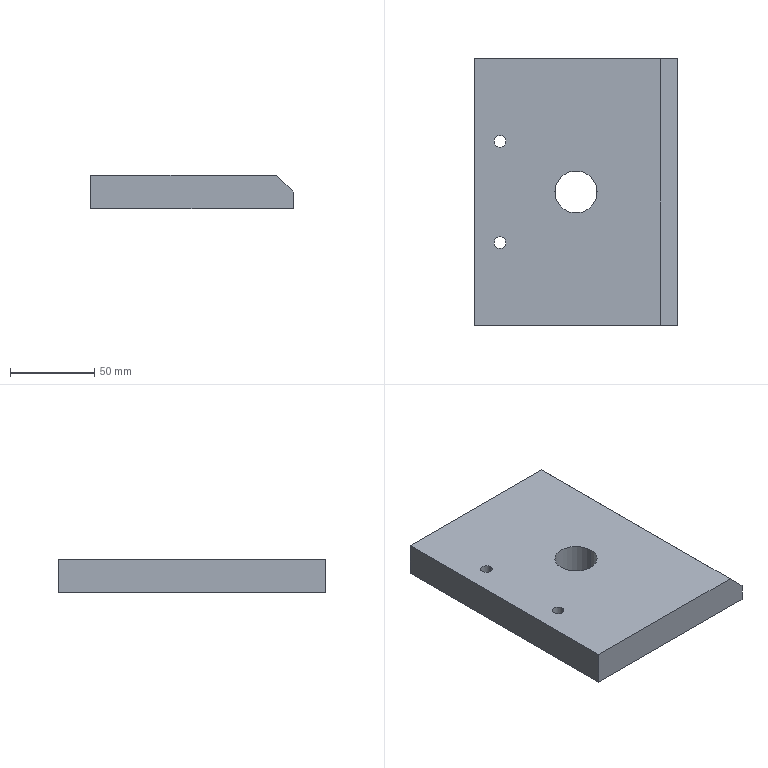Part | STEP file | 01-Top plate 1 | 1 solid | 13 faces | box 120 x 158 x 20 mm | volume 360030 mm3 | plane 7 | cylinder 6 | commonest cylinder face diameters 6.8 x4 25 x2
STEP:
#1=CARTESIAN_POINT('',(0.,0.,0.));
#2=DIRECTION('',(0.,0.,1.));
#3=DIRECTION('',(1.,0.,0.));
#4=AXIS2_PLACEMENT_3D('',#1,#2,#3);
#5=CARTESIAN_POINT('',(18.4,-49.,0.));
#6=VERTEX_POINT('',#5);
#7=CARTESIAN_POINT('',(18.4,-49.,20.));
#8=VERTEX_POINT('',#7);
#9=CARTESIAN_POINT('',(18.4,-49.,20.));
#10=DIRECTION('',(0.,0.,1.));
#11=VECTOR('',#10,1.);
#12=LINE('',#9,#11);
#13=CARTESIAN_POINT('',(15.,-49.,20.));
#14=DIRECTION('',(0.,0.,1.));
#15=DIRECTION('',(1.,0.,0.));
#16=AXIS2_PLACEMENT_3D('',#13,#14,#15);
#17=CYLINDRICAL_SURFACE('',#16,3.4);
#18=CARTESIAN_POINT('',(6.283,0.));
#19=DIRECTION('',(0.,1.));
#20=VECTOR('',#19,1.);
#21=LINE('',#18,#20);
#22=(GEOMETRIC_REPRESENTATION_CONTEXT(2)PARAMETRIC_REPRESENTATION_CONTEXT()REPRESENTATION_CONTEXT('',''));
#23=DEFINITIONAL_REPRESENTATION('',(#21),#22);
#24=PCURVE('',#17,#23);
#25=CARTESIAN_POINT('',(15.,-49.,20.));
#26=DIRECTION('',(0.,0.,1.));
#27=DIRECTION('',(1.,0.,0.));
#28=AXIS2_PLACEMENT_3D('',#25,#26,#27);
#29=CYLINDRICAL_SURFACE('',#28,3.4);
#30=CARTESIAN_POINT('',(0.,0.));
#31=DIRECTION('',(0.,1.));
#32=VECTOR('',#31,1.);
#33=LINE('',#30,#32);
#34=(GEOMETRIC_REPRESENTATION_CONTEXT(2)PARAMETRIC_REPRESENTATION_CONTEXT()REPRESENTATION_CONTEXT('',''));
#35=DEFINITIONAL_REPRESENTATION('',(#33),#34);
#36=PCURVE('',#29,#35);
#37=SURFACE_CURVE('',#12,(#24,#36),.PCURVE_S1.);
#38=EDGE_CURVE('',#6,#8,#37,.T.);
#39=ORIENTED_EDGE('',*,*,#38,.T.);
#40=CARTESIAN_POINT('',(11.6,-49.,20.));
#41=VERTEX_POINT('',#40);
#42=CARTESIAN_POINT('',(15.,-49.,20.));
#43=DIRECTION('',(0.,0.,1.));
#44=DIRECTION('',(1.,0.,0.));
#45=AXIS2_PLACEMENT_3D('',#42,#43,#44);
#46=CIRCLE('',#45,3.4);
#47=CARTESIAN_POINT('',(0.,0.));
#48=DIRECTION('',(1.,0.));
#49=VECTOR('',#48,1.);
#50=LINE('',#47,#49);
#51=(GEOMETRIC_REPRESENTATION_CONTEXT(2)PARAMETRIC_REPRESENTATION_CONTEXT()REPRESENTATION_CONTEXT('',''));
#52=DEFINITIONAL_REPRESENTATION('',(#50),#51);
#53=PCURVE('',#17,#52);
#54=CARTESIAN_POINT('',(0.,0.,20.));
#55=DIRECTION('',(0.,0.,1.));
#56=DIRECTION('',(1.,0.,0.));
#57=AXIS2_PLACEMENT_3D('',#54,#55,#56);
#58=PLANE('',#57);
#59=CARTESIAN_POINT('',(15.,-49.));
#60=DIRECTION('',(1.,0.));
#61=AXIS2_PLACEMENT_2D('',#59,#60);
#62=CIRCLE('',#61,3.4);
#63=(GEOMETRIC_REPRESENTATION_CONTEXT(2)PARAMETRIC_REPRESENTATION_CONTEXT()REPRESENTATION_CONTEXT('',''));
#64=DEFINITIONAL_REPRESENTATION('',(#62),#63);
#65=PCURVE('',#58,#64);
#66=SURFACE_CURVE('',#46,(#53,#65),.PCURVE_S1.);
#67=EDGE_CURVE('',#41,#8,#66,.T.);
#68=ORIENTED_EDGE('',*,*,#67,.F.);
#69=CARTESIAN_POINT('',(11.6,-49.,0.));
#70=VERTEX_POINT('',#69);
#71=CARTESIAN_POINT('',(11.6,-49.,20.));
#72=DIRECTION('',(0.,0.,1.));
#73=VECTOR('',#72,1.);
#74=LINE('',#71,#73);
#75=CARTESIAN_POINT('',(3.142,0.));
#76=DIRECTION('',(0.,1.));
#77=VECTOR('',#76,1.);
#78=LINE('',#75,#77);
#79=(GEOMETRIC_REPRESENTATION_CONTEXT(2)PARAMETRIC_REPRESENTATION_CONTEXT()REPRESENTATION_CONTEXT('',''));
#80=DEFINITIONAL_REPRESENTATION('',(#78),#79);
#81=PCURVE('',#17,#80);
#82=CARTESIAN_POINT('',(3.142,0.));
#83=DIRECTION('',(0.,1.));
#84=VECTOR('',#83,1.);
#85=LINE('',#82,#84);
#86=(GEOMETRIC_REPRESENTATION_CONTEXT(2)PARAMETRIC_REPRESENTATION_CONTEXT()REPRESENTATION_CONTEXT('',''));
#87=DEFINITIONAL_REPRESENTATION('',(#85),#86);
#88=PCURVE('',#29,#87);
#89=SURFACE_CURVE('',#74,(#81,#88),.PCURVE_S1.);
#90=EDGE_CURVE('',#70,#41,#89,.T.);
#91=ORIENTED_EDGE('',*,*,#90,.F.);
#92=CARTESIAN_POINT('',(15.,-49.,0.));
#93=DIRECTION('',(0.,0.,1.));
#94=DIRECTION('',(1.,0.,0.));
#95=AXIS2_PLACEMENT_3D('',#92,#93,#94);
#96=CIRCLE('',#95,3.4);
#97=CARTESIAN_POINT('',(0.,-20.));
#98=DIRECTION('',(1.,0.));
#99=VECTOR('',#98,1.);
#100=LINE('',#97,#99);
#101=(GEOMETRIC_REPRESENTATION_CONTEXT(2)PARAMETRIC_REPRESENTATION_CONTEXT()REPRESENTATION_CONTEXT('',''));
#102=DEFINITIONAL_REPRESENTATION('',(#100),#101);
#103=PCURVE('',#17,#102);
#104=CARTESIAN_POINT('',(0.,0.,0.));
#105=DIRECTION('',(0.,0.,1.));
#106=DIRECTION('',(1.,0.,0.));
#107=AXIS2_PLACEMENT_3D('',#104,#105,#106);
#108=PLANE('',#107);
#109=CARTESIAN_POINT('',(15.,-49.));
#110=DIRECTION('',(1.,0.));
#111=AXIS2_PLACEMENT_2D('',#109,#110);
#112=CIRCLE('',#111,3.4);
#113=(GEOMETRIC_REPRESENTATION_CONTEXT(2)PARAMETRIC_REPRESENTATION_CONTEXT()REPRESENTATION_CONTEXT('',''));
#114=DEFINITIONAL_REPRESENTATION('',(#112),#113);
#115=PCURVE('',#108,#114);
#116=SURFACE_CURVE('',#96,(#103,#115),.PCURVE_S1.);
#117=EDGE_CURVE('',#70,#6,#116,.T.);
#118=ORIENTED_EDGE('',*,*,#117,.T.);
#119=EDGE_LOOP('',(#39,#68,#91,#118));
#120=FACE_BOUND('',#119,.F.);
#121=ADVANCED_FACE('',(#120),#17,.F.);
#122=CARTESIAN_POINT('',(18.4,-109.,0.));
#123=VERTEX_POINT('',#122);
#124=CARTESIAN_POINT('',(18.4,-109.,20.));
#125=VERTEX_POINT('',#124);
#126=CARTESIAN_POINT('',(18.4,-109.,20.));
#127=DIRECTION('',(0.,0.,1.));
#128=VECTOR('',#127,1.);
#129=LINE('',#126,#128);
#130=CARTESIAN_POINT('',(15.,-109.,20.));
#131=DIRECTION('',(0.,0.,1.));
#132=DIRECTION('',(1.,0.,0.));
#133=AXIS2_PLACEMENT_3D('',#130,#131,#132);
#134=CYLINDRICAL_SURFACE('',#133,3.4);
#135=CARTESIAN_POINT('',(6.283,0.));
#136=DIRECTION('',(0.,1.));
#137=VECTOR('',#136,1.);
#138=LINE('',#135,#137);
#139=(GEOMETRIC_REPRESENTATION_CONTEXT(2)PARAMETRIC_REPRESENTATION_CONTEXT()REPRESENTATION_CONTEXT('',''));
#140=DEFINITIONAL_REPRESENTATION('',(#138),#139);
#141=PCURVE('',#134,#140);
#142=CARTESIAN_POINT('',(15.,-109.,20.));
#143=DIRECTION('',(0.,0.,1.));
#144=DIRECTION('',(1.,0.,0.));
#145=AXIS2_PLACEMENT_3D('',#142,#143,#144);
#146=CYLINDRICAL_SURFACE('',#145,3.4);
#147=CARTESIAN_POINT('',(0.,0.));
#148=DIRECTION('',(0.,1.));
#149=VECTOR('',#148,1.);
#150=LINE('',#147,#149);
#151=(GEOMETRIC_REPRESENTATION_CONTEXT(2)PARAMETRIC_REPRESENTATION_CONTEXT()REPRESENTATION_CONTEXT('',''));
#152=DEFINITIONAL_REPRESENTATION('',(#150),#151);
#153=PCURVE('',#146,#152);
#154=SURFACE_CURVE('',#129,(#141,#153),.PCURVE_S1.);
#155=EDGE_CURVE('',#123,#125,#154,.T.);
#156=ORIENTED_EDGE('',*,*,#155,.T.);
#157=CARTESIAN_POINT('',(11.6,-109.,20.));
#158=VERTEX_POINT('',#157);
#159=CARTESIAN_POINT('',(15.,-109.,20.));
#160=DIRECTION('',(0.,0.,1.));
#161=DIRECTION('',(1.,0.,0.));
#162=AXIS2_PLACEMENT_3D('',#159,#160,#161);
#163=CIRCLE('',#162,3.4);
#164=CARTESIAN_POINT('',(0.,0.));
#165=DIRECTION('',(1.,0.));
#166=VECTOR('',#165,1.);
#167=LINE('',#164,#166);
#168=(GEOMETRIC_REPRESENTATION_CONTEXT(2)PARAMETRIC_REPRESENTATION_CONTEXT()REPRESENTATION_CONTEXT('',''));
#169=DEFINITIONAL_REPRESENTATION('',(#167),#168);
#170=PCURVE('',#134,#169);
#171=CARTESIAN_POINT('',(15.,-109.));
#172=DIRECTION('',(1.,0.));
#173=AXIS2_PLACEMENT_2D('',#171,#172);
#174=CIRCLE('',#173,3.4);
#175=(GEOMETRIC_REPRESENTATION_CONTEXT(2)PARAMETRIC_REPRESENTATION_CONTEXT()REPRESENTATION_CONTEXT('',''));
#176=DEFINITIONAL_REPRESENTATION('',(#174),#175);
#177=PCURVE('',#58,#176);
#178=SURFACE_CURVE('',#163,(#170,#177),.PCURVE_S1.);
#179=EDGE_CURVE('',#158,#125,#178,.T.);
#180=ORIENTED_EDGE('',*,*,#179,.F.);
#181=CARTESIAN_POINT('',(11.6,-109.,0.));
#182=VERTEX_POINT('',#181);
#183=CARTESIAN_POINT('',(11.6,-109.,20.));
#184=DIRECTION('',(0.,0.,1.));
#185=VECTOR('',#184,1.);
#186=LINE('',#183,#185);
#187=CARTESIAN_POINT('',(3.142,0.));
#188=DIRECTION('',(0.,1.));
#189=VECTOR('',#188,1.);
#190=LINE('',#187,#189);
#191=(GEOMETRIC_REPRESENTATION_CONTEXT(2)PARAMETRIC_REPRESENTATION_CONTEXT()REPRESENTATION_CONTEXT('',''));
#192=DEFINITIONAL_REPRESENTATION('',(#190),#191);
#193=PCURVE('',#134,#192);
#194=CARTESIAN_POINT('',(3.142,0.));
#195=DIRECTION('',(0.,1.));
#196=VECTOR('',#195,1.);
#197=LINE('',#194,#196);
#198=(GEOMETRIC_REPRESENTATION_CONTEXT(2)PARAMETRIC_REPRESENTATION_CONTEXT()REPRESENTATION_CONTEXT('',''));
#199=DEFINITIONAL_REPRESENTATION('',(#197),#198);
#200=PCURVE('',#146,#199);
#201=SURFACE_CURVE('',#186,(#193,#200),.PCURVE_S1.);
#202=EDGE_CURVE('',#182,#158,#201,.T.);
#203=ORIENTED_EDGE('',*,*,#202,.F.);
#204=CARTESIAN_POINT('',(15.,-109.,0.));
#205=DIRECTION('',(0.,0.,1.));
#206=DIRECTION('',(1.,0.,0.));
#207=AXIS2_PLACEMENT_3D('',#204,#205,#206);
#208=CIRCLE('',#207,3.4);
#209=CARTESIAN_POINT('',(0.,-20.));
#210=DIRECTION('',(1.,0.));
#211=VECTOR('',#210,1.);
#212=LINE('',#209,#211);
#213=(GEOMETRIC_REPRESENTATION_CONTEXT(2)PARAMETRIC_REPRESENTATION_CONTEXT()REPRESENTATION_CONTEXT('',''));
#214=DEFINITIONAL_REPRESENTATION('',(#212),#213);
#215=PCURVE('',#134,#214);
#216=CARTESIAN_POINT('',(15.,-109.));
#217=DIRECTION('',(1.,0.));
#218=AXIS2_PLACEMENT_2D('',#216,#217);
#219=CIRCLE('',#218,3.4);
#220=(GEOMETRIC_REPRESENTATION_CONTEXT(2)PARAMETRIC_REPRESENTATION_CONTEXT()REPRESENTATION_CONTEXT('',''));
#221=DEFINITIONAL_REPRESENTATION('',(#219),#220);
#222=PCURVE('',#108,#221);
#223=SURFACE_CURVE('',#208,(#215,#222),.PCURVE_S1.);
#224=EDGE_CURVE('',#182,#123,#223,.T.);
#225=ORIENTED_EDGE('',*,*,#224,.T.);
#226=EDGE_LOOP('',(#156,#180,#203,#225));
#227=FACE_BOUND('',#226,.F.);
#228=ADVANCED_FACE('',(#227),#134,.F.);
#229=CARTESIAN_POINT('',(47.5,-79.,20.));
#230=VERTEX_POINT('',#229);
#231=CARTESIAN_POINT('',(47.5,-79.,0.));
#232=VERTEX_POINT('',#231);
#233=CARTESIAN_POINT('',(47.5,-79.,20.));
#234=DIRECTION('',(0.,0.,-1.));
#235=VECTOR('',#234,1.);
#236=LINE('',#233,#235);
#237=CARTESIAN_POINT('',(60.,-79.,20.));
#238=DIRECTION('',(0.,0.,-1.));
#239=DIRECTION('',(-1.,0.,0.));
#240=AXIS2_PLACEMENT_3D('',#237,#238,#239);
#241=CYLINDRICAL_SURFACE('',#240,12.5);
#242=CARTESIAN_POINT('',(6.283,0.));
#243=DIRECTION('',(0.,1.));
#244=VECTOR('',#243,1.);
#245=LINE('',#242,#244);
#246=(GEOMETRIC_REPRESENTATION_CONTEXT(2)PARAMETRIC_REPRESENTATION_CONTEXT()REPRESENTATION_CONTEXT('',''));
#247=DEFINITIONAL_REPRESENTATION('',(#245),#246);
#248=PCURVE('',#241,#247);
#249=CARTESIAN_POINT('',(60.,-79.,20.));
#250=DIRECTION('',(0.,0.,-1.));
#251=DIRECTION('',(-1.,0.,0.));
#252=AXIS2_PLACEMENT_3D('',#249,#250,#251);
#253=CYLINDRICAL_SURFACE('',#252,12.5);
#254=CARTESIAN_POINT('',(0.,0.));
#255=DIRECTION('',(0.,1.));
#256=VECTOR('',#255,1.);
#257=LINE('',#254,#256);
#258=(GEOMETRIC_REPRESENTATION_CONTEXT(2)PARAMETRIC_REPRESENTATION_CONTEXT()REPRESENTATION_CONTEXT('',''));
#259=DEFINITIONAL_REPRESENTATION('',(#257),#258);
#260=PCURVE('',#253,#259);
#261=SURFACE_CURVE('',#236,(#248,#260),.PCURVE_S1.);
#262=EDGE_CURVE('',#230,#232,#261,.T.);
#263=ORIENTED_EDGE('',*,*,#262,.T.);
#264=CARTESIAN_POINT('',(72.5,-79.,0.));
#265=VERTEX_POINT('',#264);
#266=CARTESIAN_POINT('',(60.,-79.,0.));
#267=DIRECTION('',(0.,0.,1.));
#268=DIRECTION('',(1.,0.,0.));
#269=AXIS2_PLACEMENT_3D('',#266,#267,#268);
#270=CIRCLE('',#269,12.5);
#271=CARTESIAN_POINT('',(9.425,20.));
#272=DIRECTION('',(-1.,0.));
#273=VECTOR('',#272,1.);
#274=LINE('',#271,#273);
#275=(GEOMETRIC_REPRESENTATION_CONTEXT(2)PARAMETRIC_REPRESENTATION_CONTEXT()REPRESENTATION_CONTEXT('',''));
#276=DEFINITIONAL_REPRESENTATION('',(#274),#275);
#277=PCURVE('',#241,#276);
#278=CARTESIAN_POINT('',(60.,-79.));
#279=DIRECTION('',(1.,0.));
#280=AXIS2_PLACEMENT_2D('',#278,#279);
#281=CIRCLE('',#280,12.5);
#282=(GEOMETRIC_REPRESENTATION_CONTEXT(2)PARAMETRIC_REPRESENTATION_CONTEXT()REPRESENTATION_CONTEXT('',''));
#283=DEFINITIONAL_REPRESENTATION('',(#281),#282);
#284=PCURVE('',#108,#283);
#285=SURFACE_CURVE('',#270,(#277,#284),.PCURVE_S1.);
#286=EDGE_CURVE('',#232,#265,#285,.T.);
#287=ORIENTED_EDGE('',*,*,#286,.T.);
#288=CARTESIAN_POINT('',(72.5,-79.,20.));
#289=VERTEX_POINT('',#288);
#290=CARTESIAN_POINT('',(72.5,-79.,20.));
#291=DIRECTION('',(0.,0.,-1.));
#292=VECTOR('',#291,1.);
#293=LINE('',#290,#292);
#294=CARTESIAN_POINT('',(3.142,0.));
#295=DIRECTION('',(0.,1.));
#296=VECTOR('',#295,1.);
#297=LINE('',#294,#296);
#298=(GEOMETRIC_REPRESENTATION_CONTEXT(2)PARAMETRIC_REPRESENTATION_CONTEXT()REPRESENTATION_CONTEXT('',''));
#299=DEFINITIONAL_REPRESENTATION('',(#297),#298);
#300=PCURVE('',#241,#299);
#301=CARTESIAN_POINT('',(3.142,0.));
#302=DIRECTION('',(0.,1.));
#303=VECTOR('',#302,1.);
#304=LINE('',#301,#303);
#305=(GEOMETRIC_REPRESENTATION_CONTEXT(2)PARAMETRIC_REPRESENTATION_CONTEXT()REPRESENTATION_CONTEXT('',''));
#306=DEFINITIONAL_REPRESENTATION('',(#304),#305);
#307=PCURVE('',#253,#306);
#308=SURFACE_CURVE('',#293,(#300,#307),.PCURVE_S1.);
#309=EDGE_CURVE('',#289,#265,#308,.T.);
#310=ORIENTED_EDGE('',*,*,#309,.F.);
#311=CARTESIAN_POINT('',(60.,-79.,20.));
#312=DIRECTION('',(0.,0.,1.));
#313=DIRECTION('',(1.,0.,0.));
#314=AXIS2_PLACEMENT_3D('',#311,#312,#313);
#315=CIRCLE('',#314,12.5);
#316=CARTESIAN_POINT('',(9.425,0.));
#317=DIRECTION('',(-1.,0.));
#318=VECTOR('',#317,1.);
#319=LINE('',#316,#318);
#320=(GEOMETRIC_REPRESENTATION_CONTEXT(2)PARAMETRIC_REPRESENTATION_CONTEXT()REPRESENTATION_CONTEXT('',''));
#321=DEFINITIONAL_REPRESENTATION('',(#319),#320);
#322=PCURVE('',#241,#321);
#323=CARTESIAN_POINT('',(60.,-79.));
#324=DIRECTION('',(1.,0.));
#325=AXIS2_PLACEMENT_2D('',#323,#324);
#326=CIRCLE('',#325,12.5);
#327=(GEOMETRIC_REPRESENTATION_CONTEXT(2)PARAMETRIC_REPRESENTATION_CONTEXT()REPRESENTATION_CONTEXT('',''));
#328=DEFINITIONAL_REPRESENTATION('',(#326),#327);
#329=PCURVE('',#58,#328);
#330=SURFACE_CURVE('',#315,(#322,#329),.PCURVE_S1.);
#331=EDGE_CURVE('',#230,#289,#330,.T.);
#332=ORIENTED_EDGE('',*,*,#331,.F.);
#333=EDGE_LOOP('',(#263,#287,#310,#332));
#334=FACE_BOUND('',#333,.F.);
#335=ADVANCED_FACE('',(#334),#241,.F.);
#336=CARTESIAN_POINT('',(15.,-49.,20.));
#337=DIRECTION('',(0.,0.,1.));
#338=DIRECTION('',(1.,0.,0.));
#339=AXIS2_PLACEMENT_3D('',#336,#337,#338);
#340=CIRCLE('',#339,3.4);
#341=CARTESIAN_POINT('',(15.,-49.));
#342=DIRECTION('',(1.,0.));
#343=AXIS2_PLACEMENT_2D('',#341,#342);
#344=CIRCLE('',#343,3.4);
#345=(GEOMETRIC_REPRESENTATION_CONTEXT(2)PARAMETRIC_REPRESENTATION_CONTEXT()REPRESENTATION_CONTEXT('',''));
#346=DEFINITIONAL_REPRESENTATION('',(#344),#345);
#347=PCURVE('',#58,#346);
#348=CARTESIAN_POINT('',(0.,0.));
#349=DIRECTION('',(1.,0.));
#350=VECTOR('',#349,1.);
#351=LINE('',#348,#350);
#352=(GEOMETRIC_REPRESENTATION_CONTEXT(2)PARAMETRIC_REPRESENTATION_CONTEXT()REPRESENTATION_CONTEXT('',''));
#353=DEFINITIONAL_REPRESENTATION('',(#351),#352);
#354=PCURVE('',#29,#353);
#355=SURFACE_CURVE('',#340,(#347,#354),.PCURVE_S1.);
#356=EDGE_CURVE('',#8,#41,#355,.T.);
#357=ORIENTED_EDGE('',*,*,#356,.F.);
#358=ORIENTED_EDGE('',*,*,#67,.F.);
#359=EDGE_LOOP('',(#357,#358));
#360=FACE_BOUND('',#359,.T.);
#361=CARTESIAN_POINT('',(15.,-109.,20.));
#362=DIRECTION('',(0.,0.,1.));
#363=DIRECTION('',(1.,0.,0.));
#364=AXIS2_PLACEMENT_3D('',#361,#362,#363);
#365=CIRCLE('',#364,3.4);
#366=CARTESIAN_POINT('',(15.,-109.));
#367=DIRECTION('',(1.,0.));
#368=AXIS2_PLACEMENT_2D('',#366,#367);
#369=CIRCLE('',#368,3.4);
#370=(GEOMETRIC_REPRESENTATION_CONTEXT(2)PARAMETRIC_REPRESENTATION_CONTEXT()REPRESENTATION_CONTEXT('',''));
#371=DEFINITIONAL_REPRESENTATION('',(#369),#370);
#372=PCURVE('',#58,#371);
#373=CARTESIAN_POINT('',(0.,0.));
#374=DIRECTION('',(1.,0.));
#375=VECTOR('',#374,1.);
#376=LINE('',#373,#375);
#377=(GEOMETRIC_REPRESENTATION_CONTEXT(2)PARAMETRIC_REPRESENTATION_CONTEXT()REPRESENTATION_CONTEXT('',''));
#378=DEFINITIONAL_REPRESENTATION('',(#376),#377);
#379=PCURVE('',#146,#378);
#380=SURFACE_CURVE('',#365,(#372,#379),.PCURVE_S1.);
#381=EDGE_CURVE('',#125,#158,#380,.T.);
#382=ORIENTED_EDGE('',*,*,#381,.F.);
#383=ORIENTED_EDGE('',*,*,#179,.F.);
#384=EDGE_LOOP('',(#382,#383));
#385=FACE_BOUND('',#384,.T.);
#386=CARTESIAN_POINT('',(0.,-158.,20.));
#387=VERTEX_POINT('',#386);
#388=CARTESIAN_POINT('',(110.,-158.,20.));
#389=VERTEX_POINT('',#388);
#390=CARTESIAN_POINT('',(0.,-158.,20.));
#391=DIRECTION('',(1.,0.,0.));
#392=VECTOR('',#391,1.);
#393=LINE('',#390,#392);
#394=CARTESIAN_POINT('',(0.,-158.));
#395=DIRECTION('',(1.,0.));
#396=VECTOR('',#395,1.);
#397=LINE('',#394,#396);
#398=(GEOMETRIC_REPRESENTATION_CONTEXT(2)PARAMETRIC_REPRESENTATION_CONTEXT()REPRESENTATION_CONTEXT('',''));
#399=DEFINITIONAL_REPRESENTATION('',(#397),#398);
#400=PCURVE('',#58,#399);
#401=CARTESIAN_POINT('',(0.,-158.,20.));
#402=DIRECTION('',(0.,1.,0.));
#403=DIRECTION('',(0.,0.,1.));
#404=AXIS2_PLACEMENT_3D('',#401,#402,#403);
#405=PLANE('',#404);
#406=CARTESIAN_POINT('',(0.,0.));
#407=DIRECTION('',(0.,1.));
#408=VECTOR('',#407,1.);
#409=LINE('',#406,#408);
#410=(GEOMETRIC_REPRESENTATION_CONTEXT(2)PARAMETRIC_REPRESENTATION_CONTEXT()REPRESENTATION_CONTEXT('',''));
#411=DEFINITIONAL_REPRESENTATION('',(#409),#410);
#412=PCURVE('',#405,#411);
#413=SURFACE_CURVE('',#393,(#400,#412),.PCURVE_S1.);
#414=EDGE_CURVE('',#387,#389,#413,.T.);
#415=ORIENTED_EDGE('',*,*,#414,.T.);
#416=CARTESIAN_POINT('',(110.,0.,20.));
#417=VERTEX_POINT('',#416);
#418=CARTESIAN_POINT('',(110.,0.,20.));
#419=DIRECTION('',(0.,1.,0.));
#420=VECTOR('',#419,1.);
#421=LINE('',#418,#420);
#422=CARTESIAN_POINT('',(110.,0.));
#423=DIRECTION('',(0.,1.));
#424=VECTOR('',#423,1.);
#425=LINE('',#422,#424);
#426=(GEOMETRIC_REPRESENTATION_CONTEXT(2)PARAMETRIC_REPRESENTATION_CONTEXT()REPRESENTATION_CONTEXT('',''));
#427=DEFINITIONAL_REPRESENTATION('',(#425),#426);
#428=PCURVE('',#58,#427);
#429=CARTESIAN_POINT('',(110.,0.,20.));
#430=DIRECTION('',(0.7071,0.,0.7071));
#431=DIRECTION('',(0.,-1.,0.));
#432=AXIS2_PLACEMENT_3D('',#429,#430,#431);
#433=PLANE('',#432);
#434=CARTESIAN_POINT('',(0.,0.));
#435=DIRECTION('',(-1.,0.));
#436=VECTOR('',#435,1.);
#437=LINE('',#434,#436);
#438=(GEOMETRIC_REPRESENTATION_CONTEXT(2)PARAMETRIC_REPRESENTATION_CONTEXT()REPRESENTATION_CONTEXT('',''));
#439=DEFINITIONAL_REPRESENTATION('',(#437),#438);
#440=PCURVE('',#433,#439);
#441=SURFACE_CURVE('',#421,(#428,#440),.PCURVE_S1.);
#442=EDGE_CURVE('',#389,#417,#441,.T.);
#443=ORIENTED_EDGE('',*,*,#442,.T.);
#444=CARTESIAN_POINT('',(0.,0.,20.));
#445=VERTEX_POINT('',#444);
#446=CARTESIAN_POINT('',(0.,0.,20.));
#447=DIRECTION('',(-1.,0.,0.));
#448=VECTOR('',#447,1.);
#449=LINE('',#446,#448);
#450=CARTESIAN_POINT('',(0.,0.));
#451=DIRECTION('',(-1.,0.));
#452=VECTOR('',#451,1.);
#453=LINE('',#450,#452);
#454=(GEOMETRIC_REPRESENTATION_CONTEXT(2)PARAMETRIC_REPRESENTATION_CONTEXT()REPRESENTATION_CONTEXT('',''));
#455=DEFINITIONAL_REPRESENTATION('',(#453),#454);
#456=PCURVE('',#58,#455);
#457=CARTESIAN_POINT('',(0.,0.,20.));
#458=DIRECTION('',(0.,-1.,0.));
#459=DIRECTION('',(0.,0.,-1.));
#460=AXIS2_PLACEMENT_3D('',#457,#458,#459);
#461=PLANE('',#460);
#462=CARTESIAN_POINT('',(0.,0.));
#463=DIRECTION('',(0.,-1.));
#464=VECTOR('',#463,1.);
#465=LINE('',#462,#464);
#466=(GEOMETRIC_REPRESENTATION_CONTEXT(2)PARAMETRIC_REPRESENTATION_CONTEXT()REPRESENTATION_CONTEXT('',''));
#467=DEFINITIONAL_REPRESENTATION('',(#465),#466);
#468=PCURVE('',#461,#467);
#469=SURFACE_CURVE('',#449,(#456,#468),.PCURVE_S1.);
#470=EDGE_CURVE('',#417,#445,#469,.T.);
#471=ORIENTED_EDGE('',*,*,#470,.T.);
#472=CARTESIAN_POINT('',(0.,0.,20.));
#473=DIRECTION('',(0.,-1.,0.));
#474=VECTOR('',#473,1.);
#475=LINE('',#472,#474);
#476=CARTESIAN_POINT('',(0.,0.));
#477=DIRECTION('',(0.,-1.));
#478=VECTOR('',#477,1.);
#479=LINE('',#476,#478);
#480=(GEOMETRIC_REPRESENTATION_CONTEXT(2)PARAMETRIC_REPRESENTATION_CONTEXT()REPRESENTATION_CONTEXT('',''));
#481=DEFINITIONAL_REPRESENTATION('',(#479),#480);
#482=PCURVE('',#58,#481);
#483=CARTESIAN_POINT('',(0.,0.,20.));
#484=DIRECTION('',(1.,0.,0.));
#485=DIRECTION('',(0.,1.,0.));
#486=AXIS2_PLACEMENT_3D('',#483,#484,#485);
#487=PLANE('',#486);
#488=CARTESIAN_POINT('',(0.,0.));
#489=DIRECTION('',(-1.,0.));
#490=VECTOR('',#489,1.);
#491=LINE('',#488,#490);
#492=(GEOMETRIC_REPRESENTATION_CONTEXT(2)PARAMETRIC_REPRESENTATION_CONTEXT()REPRESENTATION_CONTEXT('',''));
#493=DEFINITIONAL_REPRESENTATION('',(#491),#492);
#494=PCURVE('',#487,#493);
#495=SURFACE_CURVE('',#475,(#482,#494),.PCURVE_S1.);
#496=EDGE_CURVE('',#445,#387,#495,.T.);
#497=ORIENTED_EDGE('',*,*,#496,.T.);
#498=EDGE_LOOP('',(#415,#443,#471,#497));
#499=FACE_BOUND('',#498,.T.);
#500=ORIENTED_EDGE('',*,*,#331,.F.);
#501=CARTESIAN_POINT('',(60.,-79.,20.));
#502=DIRECTION('',(0.,0.,1.));
#503=DIRECTION('',(1.,0.,0.));
#504=AXIS2_PLACEMENT_3D('',#501,#502,#503);
#505=CIRCLE('',#504,12.5);
#506=CARTESIAN_POINT('',(60.,-79.));
#507=DIRECTION('',(1.,0.));
#508=AXIS2_PLACEMENT_2D('',#506,#507);
#509=CIRCLE('',#508,12.5);
#510=(GEOMETRIC_REPRESENTATION_CONTEXT(2)PARAMETRIC_REPRESENTATION_CONTEXT()REPRESENTATION_CONTEXT('',''));
#511=DEFINITIONAL_REPRESENTATION('',(#509),#510);
#512=PCURVE('',#58,#511);
#513=CARTESIAN_POINT('',(3.142,0.));
#514=DIRECTION('',(-1.,0.));
#515=VECTOR('',#514,1.);
#516=LINE('',#513,#515);
#517=(GEOMETRIC_REPRESENTATION_CONTEXT(2)PARAMETRIC_REPRESENTATION_CONTEXT()REPRESENTATION_CONTEXT('',''));
#518=DEFINITIONAL_REPRESENTATION('',(#516),#517);
#519=PCURVE('',#253,#518);
#520=SURFACE_CURVE('',#505,(#512,#519),.PCURVE_S1.);
#521=EDGE_CURVE('',#289,#230,#520,.T.);
#522=ORIENTED_EDGE('',*,*,#521,.F.);
#523=EDGE_LOOP('',(#500,#522));
#524=FACE_BOUND('',#523,.T.);
#525=ADVANCED_FACE('',(#360,#385,#499,#524),#58,.T.);
#526=CARTESIAN_POINT('',(15.,-49.,0.));
#527=DIRECTION('',(0.,0.,1.));
#528=DIRECTION('',(1.,0.,0.));
#529=AXIS2_PLACEMENT_3D('',#526,#527,#528);
#530=CIRCLE('',#529,3.4);
#531=CARTESIAN_POINT('',(15.,-49.));
#532=DIRECTION('',(1.,0.));
#533=AXIS2_PLACEMENT_2D('',#531,#532);
#534=CIRCLE('',#533,3.4);
#535=(GEOMETRIC_REPRESENTATION_CONTEXT(2)PARAMETRIC_REPRESENTATION_CONTEXT()REPRESENTATION_CONTEXT('',''));
#536=DEFINITIONAL_REPRESENTATION('',(#534),#535);
#537=PCURVE('',#108,#536);
#538=CARTESIAN_POINT('',(0.,-20.));
#539=DIRECTION('',(1.,0.));
#540=VECTOR('',#539,1.);
#541=LINE('',#538,#540);
#542=(GEOMETRIC_REPRESENTATION_CONTEXT(2)PARAMETRIC_REPRESENTATION_CONTEXT()REPRESENTATION_CONTEXT('',''));
#543=DEFINITIONAL_REPRESENTATION('',(#541),#542);
#544=PCURVE('',#29,#543);
#545=SURFACE_CURVE('',#530,(#537,#544),.PCURVE_S1.);
#546=EDGE_CURVE('',#6,#70,#545,.T.);
#547=ORIENTED_EDGE('',*,*,#546,.T.);
#548=ORIENTED_EDGE('',*,*,#117,.T.);
#549=EDGE_LOOP('',(#547,#548));
#550=FACE_BOUND('',#549,.T.);
#551=CARTESIAN_POINT('',(15.,-109.,0.));
#552=DIRECTION('',(0.,0.,1.));
#553=DIRECTION('',(1.,0.,0.));
#554=AXIS2_PLACEMENT_3D('',#551,#552,#553);
#555=CIRCLE('',#554,3.4);
#556=CARTESIAN_POINT('',(15.,-109.));
#557=DIRECTION('',(1.,0.));
#558=AXIS2_PLACEMENT_2D('',#556,#557);
#559=CIRCLE('',#558,3.4);
#560=(GEOMETRIC_REPRESENTATION_CONTEXT(2)PARAMETRIC_REPRESENTATION_CONTEXT()REPRESENTATION_CONTEXT('',''));
#561=DEFINITIONAL_REPRESENTATION('',(#559),#560);
#562=PCURVE('',#108,#561);
#563=CARTESIAN_POINT('',(0.,-20.));
#564=DIRECTION('',(1.,0.));
#565=VECTOR('',#564,1.);
#566=LINE('',#563,#565);
#567=(GEOMETRIC_REPRESENTATION_CONTEXT(2)PARAMETRIC_REPRESENTATION_CONTEXT()REPRESENTATION_CONTEXT('',''));
#568=DEFINITIONAL_REPRESENTATION('',(#566),#567);
#569=PCURVE('',#146,#568);
#570=SURFACE_CURVE('',#555,(#562,#569),.PCURVE_S1.);
#571=EDGE_CURVE('',#123,#182,#570,.T.);
#572=ORIENTED_EDGE('',*,*,#571,.T.);
#573=ORIENTED_EDGE('',*,*,#224,.T.);
#574=EDGE_LOOP('',(#572,#573));
#575=FACE_BOUND('',#574,.T.);
#576=CARTESIAN_POINT('',(0.,0.,0.));
#577=VERTEX_POINT('',#576);
#578=CARTESIAN_POINT('',(0.,-158.,0.));
#579=VERTEX_POINT('',#578);
#580=CARTESIAN_POINT('',(0.,0.,0.));
#581=DIRECTION('',(0.,-1.,0.));
#582=VECTOR('',#581,1.);
#583=LINE('',#580,#582);
#584=CARTESIAN_POINT('',(0.,0.));
#585=DIRECTION('',(0.,-1.));
#586=VECTOR('',#585,1.);
#587=LINE('',#584,#586);
#588=(GEOMETRIC_REPRESENTATION_CONTEXT(2)PARAMETRIC_REPRESENTATION_CONTEXT()REPRESENTATION_CONTEXT('',''));
#589=DEFINITIONAL_REPRESENTATION('',(#587),#588);
#590=PCURVE('',#108,#589);
#591=CARTESIAN_POINT('',(0.,-20.));
#592=DIRECTION('',(-1.,0.));
#593=VECTOR('',#592,1.);
#594=LINE('',#591,#593);
#595=(GEOMETRIC_REPRESENTATION_CONTEXT(2)PARAMETRIC_REPRESENTATION_CONTEXT()REPRESENTATION_CONTEXT('',''));
#596=DEFINITIONAL_REPRESENTATION('',(#594),#595);
#597=PCURVE('',#487,#596);
#598=SURFACE_CURVE('',#583,(#590,#597),.PCURVE_S1.);
#599=EDGE_CURVE('',#577,#579,#598,.T.);
#600=ORIENTED_EDGE('',*,*,#599,.F.);
#601=CARTESIAN_POINT('',(120.,0.,0.));
#602=VERTEX_POINT('',#601);
#603=CARTESIAN_POINT('',(0.,0.,0.));
#604=DIRECTION('',(-1.,0.,0.));
#605=VECTOR('',#604,1.);
#606=LINE('',#603,#605);
#607=CARTESIAN_POINT('',(0.,0.));
#608=DIRECTION('',(-1.,0.));
#609=VECTOR('',#608,1.);
#610=LINE('',#607,#609);
#611=(GEOMETRIC_REPRESENTATION_CONTEXT(2)PARAMETRIC_REPRESENTATION_CONTEXT()REPRESENTATION_CONTEXT('',''));
#612=DEFINITIONAL_REPRESENTATION('',(#610),#611);
#613=PCURVE('',#108,#612);
#614=CARTESIAN_POINT('',(20.,0.));
#615=DIRECTION('',(0.,-1.));
#616=VECTOR('',#615,1.);
#617=LINE('',#614,#616);
#618=(GEOMETRIC_REPRESENTATION_CONTEXT(2)PARAMETRIC_REPRESENTATION_CONTEXT()REPRESENTATION_CONTEXT('',''));
#619=DEFINITIONAL_REPRESENTATION('',(#617),#618);
#620=PCURVE('',#461,#619);
#621=SURFACE_CURVE('',#606,(#613,#620),.PCURVE_S1.);
#622=EDGE_CURVE('',#602,#577,#621,.T.);
#623=ORIENTED_EDGE('',*,*,#622,.F.);
#624=CARTESIAN_POINT('',(120.,-158.,0.));
#625=VERTEX_POINT('',#624);
#626=CARTESIAN_POINT('',(120.,0.,0.));
#627=DIRECTION('',(0.,1.,0.));
#628=VECTOR('',#627,1.);
#629=LINE('',#626,#628);
#630=CARTESIAN_POINT('',(120.,0.));
#631=DIRECTION('',(0.,1.));
#632=VECTOR('',#631,1.);
#633=LINE('',#630,#632);
#634=(GEOMETRIC_REPRESENTATION_CONTEXT(2)PARAMETRIC_REPRESENTATION_CONTEXT()REPRESENTATION_CONTEXT('',''));
#635=DEFINITIONAL_REPRESENTATION('',(#633),#634);
#636=PCURVE('',#108,#635);
#637=CARTESIAN_POINT('',(120.,0.,20.));
#638=DIRECTION('',(-1.,0.,0.));
#639=DIRECTION('',(0.,-1.,0.));
#640=AXIS2_PLACEMENT_3D('',#637,#638,#639);
#641=PLANE('',#640);
#642=CARTESIAN_POINT('',(0.,-20.));
#643=DIRECTION('',(-1.,0.));
#644=VECTOR('',#643,1.);
#645=LINE('',#642,#644);
#646=(GEOMETRIC_REPRESENTATION_CONTEXT(2)PARAMETRIC_REPRESENTATION_CONTEXT()REPRESENTATION_CONTEXT('',''));
#647=DEFINITIONAL_REPRESENTATION('',(#645),#646);
#648=PCURVE('',#641,#647);
#649=SURFACE_CURVE('',#629,(#636,#648),.PCURVE_S1.);
#650=EDGE_CURVE('',#625,#602,#649,.T.);
#651=ORIENTED_EDGE('',*,*,#650,.F.);
#652=CARTESIAN_POINT('',(0.,-158.,0.));
#653=DIRECTION('',(1.,0.,0.));
#654=VECTOR('',#653,1.);
#655=LINE('',#652,#654);
#656=CARTESIAN_POINT('',(0.,-158.));
#657=DIRECTION('',(1.,0.));
#658=VECTOR('',#657,1.);
#659=LINE('',#656,#658);
#660=(GEOMETRIC_REPRESENTATION_CONTEXT(2)PARAMETRIC_REPRESENTATION_CONTEXT()REPRESENTATION_CONTEXT('',''));
#661=DEFINITIONAL_REPRESENTATION('',(#659),#660);
#662=PCURVE('',#108,#661);
#663=CARTESIAN_POINT('',(-20.,0.));
#664=DIRECTION('',(0.,1.));
#665=VECTOR('',#664,1.);
#666=LINE('',#663,#665);
#667=(GEOMETRIC_REPRESENTATION_CONTEXT(2)PARAMETRIC_REPRESENTATION_CONTEXT()REPRESENTATION_CONTEXT('',''));
#668=DEFINITIONAL_REPRESENTATION('',(#666),#667);
#669=PCURVE('',#405,#668);
#670=SURFACE_CURVE('',#655,(#662,#669),.PCURVE_S1.);
#671=EDGE_CURVE('',#579,#625,#670,.T.);
#672=ORIENTED_EDGE('',*,*,#671,.F.);
#673=EDGE_LOOP('',(#600,#623,#651,#672));
#674=FACE_BOUND('',#673,.T.);
#675=ORIENTED_EDGE('',*,*,#286,.T.);
#676=CARTESIAN_POINT('',(60.,-79.,0.));
#677=DIRECTION('',(0.,0.,1.));
#678=DIRECTION('',(1.,0.,0.));
#679=AXIS2_PLACEMENT_3D('',#676,#677,#678);
#680=CIRCLE('',#679,12.5);
#681=CARTESIAN_POINT('',(60.,-79.));
#682=DIRECTION('',(1.,0.));
#683=AXIS2_PLACEMENT_2D('',#681,#682);
#684=CIRCLE('',#683,12.5);
#685=(GEOMETRIC_REPRESENTATION_CONTEXT(2)PARAMETRIC_REPRESENTATION_CONTEXT()REPRESENTATION_CONTEXT('',''));
#686=DEFINITIONAL_REPRESENTATION('',(#684),#685);
#687=PCURVE('',#108,#686);
#688=CARTESIAN_POINT('',(3.142,20.));
#689=DIRECTION('',(-1.,0.));
#690=VECTOR('',#689,1.);
#691=LINE('',#688,#690);
#692=(GEOMETRIC_REPRESENTATION_CONTEXT(2)PARAMETRIC_REPRESENTATION_CONTEXT()REPRESENTATION_CONTEXT('',''));
#693=DEFINITIONAL_REPRESENTATION('',(#691),#692);
#694=PCURVE('',#253,#693);
#695=SURFACE_CURVE('',#680,(#687,#694),.PCURVE_S1.);
#696=EDGE_CURVE('',#265,#232,#695,.T.);
#697=ORIENTED_EDGE('',*,*,#696,.T.);
#698=EDGE_LOOP('',(#675,#697));
#699=FACE_BOUND('',#698,.T.);
#700=ADVANCED_FACE('',(#550,#575,#674,#699),#108,.F.);
#701=ORIENTED_EDGE('',*,*,#599,.T.);
#702=CARTESIAN_POINT('',(0.,-158.,20.));
#703=DIRECTION('',(0.,0.,-1.));
#704=VECTOR('',#703,1.);
#705=LINE('',#702,#704);
#706=CARTESIAN_POINT('',(-158.,0.));
#707=DIRECTION('',(0.,-1.));
#708=VECTOR('',#707,1.);
#709=LINE('',#706,#708);
#710=(GEOMETRIC_REPRESENTATION_CONTEXT(2)PARAMETRIC_REPRESENTATION_CONTEXT()REPRESENTATION_CONTEXT('',''));
#711=DEFINITIONAL_REPRESENTATION('',(#709),#710);
#712=PCURVE('',#487,#711);
#713=CARTESIAN_POINT('',(0.,0.));
#714=DIRECTION('',(-1.,0.));
#715=VECTOR('',#714,1.);
#716=LINE('',#713,#715);
#717=(GEOMETRIC_REPRESENTATION_CONTEXT(2)PARAMETRIC_REPRESENTATION_CONTEXT()REPRESENTATION_CONTEXT('',''));
#718=DEFINITIONAL_REPRESENTATION('',(#716),#717);
#719=PCURVE('',#405,#718);
#720=SURFACE_CURVE('',#705,(#712,#719),.PCURVE_S1.);
#721=EDGE_CURVE('',#387,#579,#720,.T.);
#722=ORIENTED_EDGE('',*,*,#721,.F.);
#723=ORIENTED_EDGE('',*,*,#496,.F.);
#724=CARTESIAN_POINT('',(0.,0.,20.));
#725=DIRECTION('',(0.,0.,-1.));
#726=VECTOR('',#725,1.);
#727=LINE('',#724,#726);
#728=CARTESIAN_POINT('',(0.,0.));
#729=DIRECTION('',(0.,-1.));
#730=VECTOR('',#729,1.);
#731=LINE('',#728,#730);
#732=(GEOMETRIC_REPRESENTATION_CONTEXT(2)PARAMETRIC_REPRESENTATION_CONTEXT()REPRESENTATION_CONTEXT('',''));
#733=DEFINITIONAL_REPRESENTATION('',(#731),#732);
#734=PCURVE('',#487,#733);
#735=CARTESIAN_POINT('',(0.,0.));
#736=DIRECTION('',(1.,0.));
#737=VECTOR('',#736,1.);
#738=LINE('',#735,#737);
#739=(GEOMETRIC_REPRESENTATION_CONTEXT(2)PARAMETRIC_REPRESENTATION_CONTEXT()REPRESENTATION_CONTEXT('',''));
#740=DEFINITIONAL_REPRESENTATION('',(#738),#739);
#741=PCURVE('',#461,#740);
#742=SURFACE_CURVE('',#727,(#734,#741),.PCURVE_S1.);
#743=EDGE_CURVE('',#445,#577,#742,.T.);
#744=ORIENTED_EDGE('',*,*,#743,.T.);
#745=EDGE_LOOP('',(#701,#722,#723,#744));
#746=FACE_BOUND('',#745,.T.);
#747=ADVANCED_FACE('',(#746),#487,.F.);
#748=CARTESIAN_POINT('',(120.,-158.,10.));
#749=VERTEX_POINT('',#748);
#750=CARTESIAN_POINT('',(120.,-158.,20.));
#751=DIRECTION('',(0.,0.,-1.));
#752=VECTOR('',#751,1.);
#753=LINE('',#750,#752);
#754=CARTESIAN_POINT('',(0.,120.));
#755=DIRECTION('',(-1.,0.));
#756=VECTOR('',#755,1.);
#757=LINE('',#754,#756);
#758=(GEOMETRIC_REPRESENTATION_CONTEXT(2)PARAMETRIC_REPRESENTATION_CONTEXT()REPRESENTATION_CONTEXT('',''));
#759=DEFINITIONAL_REPRESENTATION('',(#757),#758);
#760=PCURVE('',#405,#759);
#761=CARTESIAN_POINT('',(158.,0.));
#762=DIRECTION('',(0.,-1.));
#763=VECTOR('',#762,1.);
#764=LINE('',#761,#763);
#765=(GEOMETRIC_REPRESENTATION_CONTEXT(2)PARAMETRIC_REPRESENTATION_CONTEXT()REPRESENTATION_CONTEXT('',''));
#766=DEFINITIONAL_REPRESENTATION('',(#764),#765);
#767=PCURVE('',#641,#766);
#768=SURFACE_CURVE('',#753,(#760,#767),.PCURVE_S1.);
#769=EDGE_CURVE('',#749,#625,#768,.T.);
#770=ORIENTED_EDGE('',*,*,#769,.F.);
#771=CARTESIAN_POINT('',(110.,-158.,20.));
#772=DIRECTION('',(-0.7071,0.,0.7071));
#773=VECTOR('',#772,1.);
#774=LINE('',#771,#773);
#775=CARTESIAN_POINT('',(0.,110.));
#776=DIRECTION('',(0.7071,-0.7071));
#777=VECTOR('',#776,1.);
#778=LINE('',#775,#777);
#779=(GEOMETRIC_REPRESENTATION_CONTEXT(2)PARAMETRIC_REPRESENTATION_CONTEXT()REPRESENTATION_CONTEXT('',''));
#780=DEFINITIONAL_REPRESENTATION('',(#778),#779);
#781=PCURVE('',#405,#780);
#782=CARTESIAN_POINT('',(158.,0.));
#783=DIRECTION('',(0.,-1.));
#784=VECTOR('',#783,1.);
#785=LINE('',#782,#784);
#786=(GEOMETRIC_REPRESENTATION_CONTEXT(2)PARAMETRIC_REPRESENTATION_CONTEXT()REPRESENTATION_CONTEXT('',''));
#787=DEFINITIONAL_REPRESENTATION('',(#785),#786);
#788=PCURVE('',#433,#787);
#789=SURFACE_CURVE('',#774,(#781,#788),.PCURVE_S1.);
#790=EDGE_CURVE('',#749,#389,#789,.T.);
#791=ORIENTED_EDGE('',*,*,#790,.T.);
#792=ORIENTED_EDGE('',*,*,#414,.F.);
#793=ORIENTED_EDGE('',*,*,#721,.T.);
#794=ORIENTED_EDGE('',*,*,#671,.T.);
#795=EDGE_LOOP('',(#770,#791,#792,#793,#794));
#796=FACE_BOUND('',#795,.T.);
#797=ADVANCED_FACE('',(#796),#405,.F.);
#798=CARTESIAN_POINT('',(120.,0.,10.));
#799=VERTEX_POINT('',#798);
#800=CARTESIAN_POINT('',(120.,0.,20.));
#801=DIRECTION('',(0.,0.,-1.));
#802=VECTOR('',#801,1.);
#803=LINE('',#800,#802);
#804=CARTESIAN_POINT('',(0.,0.));
#805=DIRECTION('',(0.,-1.));
#806=VECTOR('',#805,1.);
#807=LINE('',#804,#806);
#808=(GEOMETRIC_REPRESENTATION_CONTEXT(2)PARAMETRIC_REPRESENTATION_CONTEXT()REPRESENTATION_CONTEXT('',''));
#809=DEFINITIONAL_REPRESENTATION('',(#807),#808);
#810=PCURVE('',#641,#809);
#811=CARTESIAN_POINT('',(0.,120.));
#812=DIRECTION('',(1.,0.));
#813=VECTOR('',#812,1.);
#814=LINE('',#811,#813);
#815=(GEOMETRIC_REPRESENTATION_CONTEXT(2)PARAMETRIC_REPRESENTATION_CONTEXT()REPRESENTATION_CONTEXT('',''));
#816=DEFINITIONAL_REPRESENTATION('',(#814),#815);
#817=PCURVE('',#461,#816);
#818=SURFACE_CURVE('',#803,(#810,#817),.PCURVE_S1.);
#819=EDGE_CURVE('',#799,#602,#818,.T.);
#820=ORIENTED_EDGE('',*,*,#819,.F.);
#821=CARTESIAN_POINT('',(120.,-158.,10.));
#822=DIRECTION('',(0.,-1.,0.));
#823=VECTOR('',#822,1.);
#824=LINE('',#821,#823);
#825=CARTESIAN_POINT('',(158.,-10.));
#826=DIRECTION('',(1.,0.));
#827=VECTOR('',#826,1.);
#828=LINE('',#825,#827);
#829=(GEOMETRIC_REPRESENTATION_CONTEXT(2)PARAMETRIC_REPRESENTATION_CONTEXT()REPRESENTATION_CONTEXT('',''));
#830=DEFINITIONAL_REPRESENTATION('',(#828),#829);
#831=PCURVE('',#641,#830);
#832=CARTESIAN_POINT('',(158.,14.142));
#833=DIRECTION('',(1.,0.));
#834=VECTOR('',#833,1.);
#835=LINE('',#832,#834);
#836=(GEOMETRIC_REPRESENTATION_CONTEXT(2)PARAMETRIC_REPRESENTATION_CONTEXT()REPRESENTATION_CONTEXT('',''));
#837=DEFINITIONAL_REPRESENTATION('',(#835),#836);
#838=PCURVE('',#433,#837);
#839=SURFACE_CURVE('',#824,(#831,#838),.PCURVE_S1.);
#840=EDGE_CURVE('',#799,#749,#839,.T.);
#841=ORIENTED_EDGE('',*,*,#840,.T.);
#842=ORIENTED_EDGE('',*,*,#769,.T.);
#843=ORIENTED_EDGE('',*,*,#650,.T.);
#844=EDGE_LOOP('',(#820,#841,#842,#843));
#845=FACE_BOUND('',#844,.T.);
#846=ADVANCED_FACE('',(#845),#641,.F.);
#847=ORIENTED_EDGE('',*,*,#470,.F.);
#848=CARTESIAN_POINT('',(110.,0.,20.));
#849=DIRECTION('',(0.7071,0.,-0.7071));
#850=VECTOR('',#849,1.);
#851=LINE('',#848,#850);
#852=CARTESIAN_POINT('',(0.,110.));
#853=DIRECTION('',(0.7071,0.7071));
#854=VECTOR('',#853,1.);
#855=LINE('',#852,#854);
#856=(GEOMETRIC_REPRESENTATION_CONTEXT(2)PARAMETRIC_REPRESENTATION_CONTEXT()REPRESENTATION_CONTEXT('',''));
#857=DEFINITIONAL_REPRESENTATION('',(#855),#856);
#858=PCURVE('',#461,#857);
#859=CARTESIAN_POINT('',(0.,0.));
#860=DIRECTION('',(0.,1.));
#861=VECTOR('',#860,1.);
#862=LINE('',#859,#861);
#863=(GEOMETRIC_REPRESENTATION_CONTEXT(2)PARAMETRIC_REPRESENTATION_CONTEXT()REPRESENTATION_CONTEXT('',''));
#864=DEFINITIONAL_REPRESENTATION('',(#862),#863);
#865=PCURVE('',#433,#864);
#866=SURFACE_CURVE('',#851,(#858,#865),.PCURVE_S1.);
#867=EDGE_CURVE('',#417,#799,#866,.T.);
#868=ORIENTED_EDGE('',*,*,#867,.T.);
#869=ORIENTED_EDGE('',*,*,#819,.T.);
#870=ORIENTED_EDGE('',*,*,#622,.T.);
#871=ORIENTED_EDGE('',*,*,#743,.F.);
#872=EDGE_LOOP('',(#847,#868,#869,#870,#871));
#873=FACE_BOUND('',#872,.T.);
#874=ADVANCED_FACE('',(#873),#461,.F.);
#875=ORIENTED_EDGE('',*,*,#696,.T.);
#876=ORIENTED_EDGE('',*,*,#262,.F.);
#877=ORIENTED_EDGE('',*,*,#521,.F.);
#878=ORIENTED_EDGE('',*,*,#309,.T.);
#879=EDGE_LOOP('',(#875,#876,#877,#878));
#880=FACE_BOUND('',#879,.F.);
#881=ADVANCED_FACE('',(#880),#253,.F.);
#882=ORIENTED_EDGE('',*,*,#790,.F.);
#883=ORIENTED_EDGE('',*,*,#840,.F.);
#884=ORIENTED_EDGE('',*,*,#867,.F.);
#885=ORIENTED_EDGE('',*,*,#442,.F.);
#886=EDGE_LOOP('',(#882,#883,#884,#885));
#887=FACE_BOUND('',#886,.T.);
#888=ADVANCED_FACE('',(#887),#433,.T.);
#889=ORIENTED_EDGE('',*,*,#381,.F.);
#890=ORIENTED_EDGE('',*,*,#155,.F.);
#891=ORIENTED_EDGE('',*,*,#571,.T.);
#892=ORIENTED_EDGE('',*,*,#202,.T.);
#893=EDGE_LOOP('',(#889,#890,#891,#892));
#894=FACE_BOUND('',#893,.F.);
#895=ADVANCED_FACE('',(#894),#146,.F.);
#896=ORIENTED_EDGE('',*,*,#356,.F.);
#897=ORIENTED_EDGE('',*,*,#38,.F.);
#898=ORIENTED_EDGE('',*,*,#546,.T.);
#899=ORIENTED_EDGE('',*,*,#90,.T.);
#900=EDGE_LOOP('',(#896,#897,#898,#899));
#901=FACE_BOUND('',#900,.F.);
#902=ADVANCED_FACE('',(#901),#29,.F.);
#903=CLOSED_SHELL('',(#121,#228,#335,#525,#700,#747,#797,#846,#874,#881,#888,#895,#902));
#904=MANIFOLD_SOLID_BREP('',#903);
#905=(LENGTH_UNIT()NAMED_UNIT(*)SI_UNIT(.MILLI.,.METRE.));
#906=UNCERTAINTY_MEASURE_WITH_UNIT(LENGTH_MEASURE(0.0000001),#905,'','');
#907=(NAMED_UNIT(*)PLANE_ANGLE_UNIT()SI_UNIT($,.RADIAN.));
#908=(NAMED_UNIT(*)SI_UNIT($,.STERADIAN.)SOLID_ANGLE_UNIT());
#909=(GEOMETRIC_REPRESENTATION_CONTEXT(3)GLOBAL_UNCERTAINTY_ASSIGNED_CONTEXT((#906))GLOBAL_UNIT_ASSIGNED_CONTEXT((#905,#907,#908))REPRESENTATION_CONTEXT('',''));
#910=ADVANCED_BREP_SHAPE_REPRESENTATION('',(#4,#904),#909);